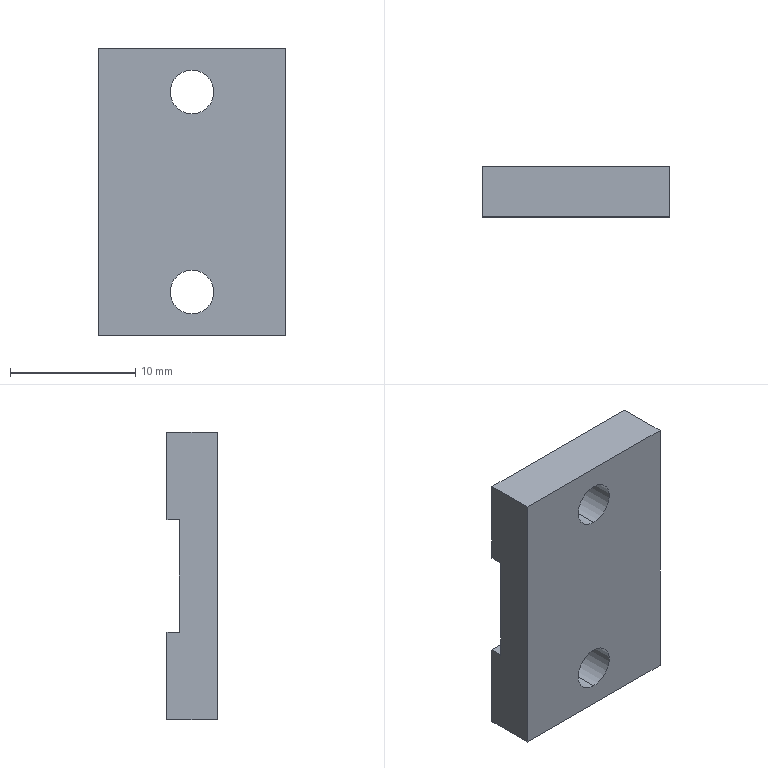Part | STEP file | 06-26 Cutter press block | 1 solid | 14 faces | box 15 x 4 x 23 mm | volume 1168 mm3 | plane 10 | cylinder 4 | commonest cylinder face diameters 3.5 x4
STEP:
#1=CARTESIAN_POINT('',(0.,0.,0.));
#2=DIRECTION('',(0.,0.,1.));
#3=DIRECTION('',(1.,0.,0.));
#4=AXIS2_PLACEMENT_3D('',#1,#2,#3);
#5=CARTESIAN_POINT('',(0.,4.,6.25));
#6=VERTEX_POINT('',#5);
#7=CARTESIAN_POINT('',(0.,0.,6.25));
#8=VERTEX_POINT('',#7);
#9=CARTESIAN_POINT('',(0.,4.,6.25));
#10=DIRECTION('',(0.,-1.,0.));
#11=VECTOR('',#10,1.);
#12=LINE('',#9,#11);
#13=CARTESIAN_POINT('',(0.,4.,8.));
#14=DIRECTION('',(0.,-1.,0.));
#15=DIRECTION('',(0.,0.,-1.));
#16=AXIS2_PLACEMENT_3D('',#13,#14,#15);
#17=CYLINDRICAL_SURFACE('',#16,1.75);
#18=CARTESIAN_POINT('',(6.283,0.));
#19=DIRECTION('',(0.,1.));
#20=VECTOR('',#19,1.);
#21=LINE('',#18,#20);
#22=(GEOMETRIC_REPRESENTATION_CONTEXT(2)PARAMETRIC_REPRESENTATION_CONTEXT()REPRESENTATION_CONTEXT('',''));
#23=DEFINITIONAL_REPRESENTATION('',(#21),#22);
#24=PCURVE('',#17,#23);
#25=CARTESIAN_POINT('',(0.,4.,8.));
#26=DIRECTION('',(0.,-1.,0.));
#27=DIRECTION('',(0.,0.,-1.));
#28=AXIS2_PLACEMENT_3D('',#25,#26,#27);
#29=CYLINDRICAL_SURFACE('',#28,1.75);
#30=CARTESIAN_POINT('',(0.,0.));
#31=DIRECTION('',(0.,1.));
#32=VECTOR('',#31,1.);
#33=LINE('',#30,#32);
#34=(GEOMETRIC_REPRESENTATION_CONTEXT(2)PARAMETRIC_REPRESENTATION_CONTEXT()REPRESENTATION_CONTEXT('',''));
#35=DEFINITIONAL_REPRESENTATION('',(#33),#34);
#36=PCURVE('',#29,#35);
#37=SURFACE_CURVE('',#12,(#24,#36),.PCURVE_S1.);
#38=EDGE_CURVE('',#6,#8,#37,.T.);
#39=ORIENTED_EDGE('',*,*,#38,.T.);
#40=CARTESIAN_POINT('',(0.,0.,9.75));
#41=VERTEX_POINT('',#40);
#42=CARTESIAN_POINT('',(0.,0.,8.));
#43=DIRECTION('',(0.,-1.,0.));
#44=DIRECTION('',(0.,0.,-1.));
#45=AXIS2_PLACEMENT_3D('',#42,#43,#44);
#46=CIRCLE('',#45,1.75);
#47=CARTESIAN_POINT('',(0.,4.));
#48=DIRECTION('',(1.,0.));
#49=VECTOR('',#48,1.);
#50=LINE('',#47,#49);
#51=(GEOMETRIC_REPRESENTATION_CONTEXT(2)PARAMETRIC_REPRESENTATION_CONTEXT()REPRESENTATION_CONTEXT('',''));
#52=DEFINITIONAL_REPRESENTATION('',(#50),#51);
#53=PCURVE('',#17,#52);
#54=CARTESIAN_POINT('',(-7.5,0.,-11.5));
#55=DIRECTION('',(0.,1.,0.));
#56=DIRECTION('',(0.,0.,1.));
#57=AXIS2_PLACEMENT_3D('',#54,#55,#56);
#58=PLANE('',#57);
#59=CARTESIAN_POINT('',(17.75,7.5));
#60=CARTESIAN_POINT('',(17.75,10.531));
#61=CARTESIAN_POINT('',(20.375,9.016));
#62=CARTESIAN_POINT('',(23.,7.5));
#63=CARTESIAN_POINT('',(20.375,5.984));
#64=CARTESIAN_POINT('',(17.75,4.469));
#65=CARTESIAN_POINT('',(17.75,7.5));
#66=(BOUNDED_CURVE()B_SPLINE_CURVE(2,(#59,#60,#61,#62,#63,#64,#65),.UNSPECIFIED.,.T.,.F.)B_SPLINE_CURVE_WITH_KNOTS((1,2,2,2,2,1),(-2.094,0.,2.094,4.189,6.283,8.378),.UNSPECIFIED.)CURVE()GEOMETRIC_REPRESENTATION_ITEM()RATIONAL_B_SPLINE_CURVE((1.,0.5,1.,0.5,1.,0.5,1.))REPRESENTATION_ITEM(''));
#67=(GEOMETRIC_REPRESENTATION_CONTEXT(2)PARAMETRIC_REPRESENTATION_CONTEXT()REPRESENTATION_CONTEXT('',''));
#68=DEFINITIONAL_REPRESENTATION('',(#66),#67);
#69=PCURVE('',#58,#68);
#70=SURFACE_CURVE('',#46,(#53,#69),.PCURVE_S1.);
#71=EDGE_CURVE('',#41,#8,#70,.T.);
#72=ORIENTED_EDGE('',*,*,#71,.F.);
#73=CARTESIAN_POINT('',(0.,4.,9.75));
#74=VERTEX_POINT('',#73);
#75=CARTESIAN_POINT('',(0.,4.,9.75));
#76=DIRECTION('',(0.,-1.,0.));
#77=VECTOR('',#76,1.);
#78=LINE('',#75,#77);
#79=CARTESIAN_POINT('',(3.142,0.));
#80=DIRECTION('',(0.,1.));
#81=VECTOR('',#80,1.);
#82=LINE('',#79,#81);
#83=(GEOMETRIC_REPRESENTATION_CONTEXT(2)PARAMETRIC_REPRESENTATION_CONTEXT()REPRESENTATION_CONTEXT('',''));
#84=DEFINITIONAL_REPRESENTATION('',(#82),#83);
#85=PCURVE('',#17,#84);
#86=CARTESIAN_POINT('',(3.142,0.));
#87=DIRECTION('',(0.,1.));
#88=VECTOR('',#87,1.);
#89=LINE('',#86,#88);
#90=(GEOMETRIC_REPRESENTATION_CONTEXT(2)PARAMETRIC_REPRESENTATION_CONTEXT()REPRESENTATION_CONTEXT('',''));
#91=DEFINITIONAL_REPRESENTATION('',(#89),#90);
#92=PCURVE('',#29,#91);
#93=SURFACE_CURVE('',#78,(#85,#92),.PCURVE_S1.);
#94=EDGE_CURVE('',#74,#41,#93,.T.);
#95=ORIENTED_EDGE('',*,*,#94,.F.);
#96=CARTESIAN_POINT('',(0.,4.,8.));
#97=DIRECTION('',(0.,1.,0.));
#98=DIRECTION('',(0.,0.,-1.));
#99=AXIS2_PLACEMENT_3D('',#96,#97,#98);
#100=CIRCLE('',#99,1.75);
#101=CARTESIAN_POINT('',(6.283,0.));
#102=DIRECTION('',(-1.,0.));
#103=VECTOR('',#102,1.);
#104=LINE('',#101,#103);
#105=(GEOMETRIC_REPRESENTATION_CONTEXT(2)PARAMETRIC_REPRESENTATION_CONTEXT()REPRESENTATION_CONTEXT('',''));
#106=DEFINITIONAL_REPRESENTATION('',(#104),#105);
#107=PCURVE('',#17,#106);
#108=CARTESIAN_POINT('',(-7.5,4.,11.5));
#109=DIRECTION('',(0.,-1.,0.));
#110=DIRECTION('',(0.,0.,-1.));
#111=AXIS2_PLACEMENT_3D('',#108,#109,#110);
#112=PLANE('',#111);
#113=CARTESIAN_POINT('',(5.25,7.5));
#114=CARTESIAN_POINT('',(5.25,4.469));
#115=CARTESIAN_POINT('',(2.625,5.984));
#116=CARTESIAN_POINT('',(0.,7.5));
#117=CARTESIAN_POINT('',(2.625,9.016));
#118=CARTESIAN_POINT('',(5.25,10.531));
#119=CARTESIAN_POINT('',(5.25,7.5));
#120=(BOUNDED_CURVE()B_SPLINE_CURVE(2,(#113,#114,#115,#116,#117,#118,#119),.UNSPECIFIED.,.T.,.F.)B_SPLINE_CURVE_WITH_KNOTS((1,2,2,2,2,1),(-2.094,0.,2.094,4.189,6.283,8.378),.UNSPECIFIED.)CURVE()GEOMETRIC_REPRESENTATION_ITEM()RATIONAL_B_SPLINE_CURVE((1.,0.5,1.,0.5,1.,0.5,1.))REPRESENTATION_ITEM(''));
#121=(GEOMETRIC_REPRESENTATION_CONTEXT(2)PARAMETRIC_REPRESENTATION_CONTEXT()REPRESENTATION_CONTEXT('',''));
#122=DEFINITIONAL_REPRESENTATION('',(#120),#121);
#123=PCURVE('',#112,#122);
#124=SURFACE_CURVE('',#100,(#107,#123),.PCURVE_S1.);
#125=EDGE_CURVE('',#6,#74,#124,.T.);
#126=ORIENTED_EDGE('',*,*,#125,.F.);
#127=EDGE_LOOP('',(#39,#72,#95,#126));
#128=FACE_BOUND('',#127,.F.);
#129=ADVANCED_FACE('',(#128),#17,.F.);
#130=CARTESIAN_POINT('',(0.,4.,-9.75));
#131=VERTEX_POINT('',#130);
#132=CARTESIAN_POINT('',(0.,0.,-9.75));
#133=VERTEX_POINT('',#132);
#134=CARTESIAN_POINT('',(0.,4.,-9.75));
#135=DIRECTION('',(0.,-1.,0.));
#136=VECTOR('',#135,1.);
#137=LINE('',#134,#136);
#138=CARTESIAN_POINT('',(0.,4.,-8.));
#139=DIRECTION('',(0.,-1.,0.));
#140=DIRECTION('',(0.,0.,-1.));
#141=AXIS2_PLACEMENT_3D('',#138,#139,#140);
#142=CYLINDRICAL_SURFACE('',#141,1.75);
#143=CARTESIAN_POINT('',(6.283,0.));
#144=DIRECTION('',(0.,1.));
#145=VECTOR('',#144,1.);
#146=LINE('',#143,#145);
#147=(GEOMETRIC_REPRESENTATION_CONTEXT(2)PARAMETRIC_REPRESENTATION_CONTEXT()REPRESENTATION_CONTEXT('',''));
#148=DEFINITIONAL_REPRESENTATION('',(#146),#147);
#149=PCURVE('',#142,#148);
#150=CARTESIAN_POINT('',(0.,4.,-8.));
#151=DIRECTION('',(0.,-1.,0.));
#152=DIRECTION('',(0.,0.,-1.));
#153=AXIS2_PLACEMENT_3D('',#150,#151,#152);
#154=CYLINDRICAL_SURFACE('',#153,1.75);
#155=CARTESIAN_POINT('',(0.,0.));
#156=DIRECTION('',(0.,1.));
#157=VECTOR('',#156,1.);
#158=LINE('',#155,#157);
#159=(GEOMETRIC_REPRESENTATION_CONTEXT(2)PARAMETRIC_REPRESENTATION_CONTEXT()REPRESENTATION_CONTEXT('',''));
#160=DEFINITIONAL_REPRESENTATION('',(#158),#159);
#161=PCURVE('',#154,#160);
#162=SURFACE_CURVE('',#137,(#149,#161),.PCURVE_S1.);
#163=EDGE_CURVE('',#131,#133,#162,.T.);
#164=ORIENTED_EDGE('',*,*,#163,.T.);
#165=CARTESIAN_POINT('',(0.,0.,-6.25));
#166=VERTEX_POINT('',#165);
#167=CARTESIAN_POINT('',(0.,0.,-8.));
#168=DIRECTION('',(0.,-1.,0.));
#169=DIRECTION('',(0.,0.,-1.));
#170=AXIS2_PLACEMENT_3D('',#167,#168,#169);
#171=CIRCLE('',#170,1.75);
#172=CARTESIAN_POINT('',(0.,4.));
#173=DIRECTION('',(1.,0.));
#174=VECTOR('',#173,1.);
#175=LINE('',#172,#174);
#176=(GEOMETRIC_REPRESENTATION_CONTEXT(2)PARAMETRIC_REPRESENTATION_CONTEXT()REPRESENTATION_CONTEXT('',''));
#177=DEFINITIONAL_REPRESENTATION('',(#175),#176);
#178=PCURVE('',#142,#177);
#179=CARTESIAN_POINT('',(1.75,7.5));
#180=CARTESIAN_POINT('',(1.75,10.531));
#181=CARTESIAN_POINT('',(4.375,9.016));
#182=CARTESIAN_POINT('',(7.,7.5));
#183=CARTESIAN_POINT('',(4.375,5.984));
#184=CARTESIAN_POINT('',(1.75,4.469));
#185=CARTESIAN_POINT('',(1.75,7.5));
#186=(BOUNDED_CURVE()B_SPLINE_CURVE(2,(#179,#180,#181,#182,#183,#184,#185),.UNSPECIFIED.,.T.,.F.)B_SPLINE_CURVE_WITH_KNOTS((1,2,2,2,2,1),(-2.094,0.,2.094,4.189,6.283,8.378),.UNSPECIFIED.)CURVE()GEOMETRIC_REPRESENTATION_ITEM()RATIONAL_B_SPLINE_CURVE((1.,0.5,1.,0.5,1.,0.5,1.))REPRESENTATION_ITEM(''));
#187=(GEOMETRIC_REPRESENTATION_CONTEXT(2)PARAMETRIC_REPRESENTATION_CONTEXT()REPRESENTATION_CONTEXT('',''));
#188=DEFINITIONAL_REPRESENTATION('',(#186),#187);
#189=PCURVE('',#58,#188);
#190=SURFACE_CURVE('',#171,(#178,#189),.PCURVE_S1.);
#191=EDGE_CURVE('',#166,#133,#190,.T.);
#192=ORIENTED_EDGE('',*,*,#191,.F.);
#193=CARTESIAN_POINT('',(0.,4.,-6.25));
#194=VERTEX_POINT('',#193);
#195=CARTESIAN_POINT('',(0.,4.,-6.25));
#196=DIRECTION('',(0.,-1.,0.));
#197=VECTOR('',#196,1.);
#198=LINE('',#195,#197);
#199=CARTESIAN_POINT('',(3.142,0.));
#200=DIRECTION('',(0.,1.));
#201=VECTOR('',#200,1.);
#202=LINE('',#199,#201);
#203=(GEOMETRIC_REPRESENTATION_CONTEXT(2)PARAMETRIC_REPRESENTATION_CONTEXT()REPRESENTATION_CONTEXT('',''));
#204=DEFINITIONAL_REPRESENTATION('',(#202),#203);
#205=PCURVE('',#142,#204);
#206=CARTESIAN_POINT('',(3.142,0.));
#207=DIRECTION('',(0.,1.));
#208=VECTOR('',#207,1.);
#209=LINE('',#206,#208);
#210=(GEOMETRIC_REPRESENTATION_CONTEXT(2)PARAMETRIC_REPRESENTATION_CONTEXT()REPRESENTATION_CONTEXT('',''));
#211=DEFINITIONAL_REPRESENTATION('',(#209),#210);
#212=PCURVE('',#154,#211);
#213=SURFACE_CURVE('',#198,(#205,#212),.PCURVE_S1.);
#214=EDGE_CURVE('',#194,#166,#213,.T.);
#215=ORIENTED_EDGE('',*,*,#214,.F.);
#216=CARTESIAN_POINT('',(0.,4.,-8.));
#217=DIRECTION('',(0.,1.,0.));
#218=DIRECTION('',(0.,0.,-1.));
#219=AXIS2_PLACEMENT_3D('',#216,#217,#218);
#220=CIRCLE('',#219,1.75);
#221=CARTESIAN_POINT('',(6.283,0.));
#222=DIRECTION('',(-1.,0.));
#223=VECTOR('',#222,1.);
#224=LINE('',#221,#223);
#225=(GEOMETRIC_REPRESENTATION_CONTEXT(2)PARAMETRIC_REPRESENTATION_CONTEXT()REPRESENTATION_CONTEXT('',''));
#226=DEFINITIONAL_REPRESENTATION('',(#224),#225);
#227=PCURVE('',#142,#226);
#228=CARTESIAN_POINT('',(-7.5,4.,-4.5));
#229=DIRECTION('',(0.,-1.,0.));
#230=DIRECTION('',(0.,0.,-1.));
#231=AXIS2_PLACEMENT_3D('',#228,#229,#230);
#232=PLANE('',#231);
#233=CARTESIAN_POINT('',(5.25,7.5));
#234=CARTESIAN_POINT('',(5.25,4.469));
#235=CARTESIAN_POINT('',(2.625,5.984));
#236=CARTESIAN_POINT('',(0.,7.5));
#237=CARTESIAN_POINT('',(2.625,9.016));
#238=CARTESIAN_POINT('',(5.25,10.531));
#239=CARTESIAN_POINT('',(5.25,7.5));
#240=(BOUNDED_CURVE()B_SPLINE_CURVE(2,(#233,#234,#235,#236,#237,#238,#239),.UNSPECIFIED.,.T.,.F.)B_SPLINE_CURVE_WITH_KNOTS((1,2,2,2,2,1),(-2.094,0.,2.094,4.189,6.283,8.378),.UNSPECIFIED.)CURVE()GEOMETRIC_REPRESENTATION_ITEM()RATIONAL_B_SPLINE_CURVE((1.,0.5,1.,0.5,1.,0.5,1.))REPRESENTATION_ITEM(''));
#241=(GEOMETRIC_REPRESENTATION_CONTEXT(2)PARAMETRIC_REPRESENTATION_CONTEXT()REPRESENTATION_CONTEXT('',''));
#242=DEFINITIONAL_REPRESENTATION('',(#240),#241);
#243=PCURVE('',#232,#242);
#244=SURFACE_CURVE('',#220,(#227,#243),.PCURVE_S1.);
#245=EDGE_CURVE('',#131,#194,#244,.T.);
#246=ORIENTED_EDGE('',*,*,#245,.F.);
#247=EDGE_LOOP('',(#164,#192,#215,#246));
#248=FACE_BOUND('',#247,.F.);
#249=ADVANCED_FACE('',(#248),#142,.F.);
#250=CARTESIAN_POINT('',(0.,0.,8.));
#251=DIRECTION('',(0.,-1.,0.));
#252=DIRECTION('',(0.,0.,-1.));
#253=AXIS2_PLACEMENT_3D('',#250,#251,#252);
#254=CIRCLE('',#253,1.75);
#255=CARTESIAN_POINT('',(0.,4.));
#256=DIRECTION('',(1.,0.));
#257=VECTOR('',#256,1.);
#258=LINE('',#255,#257);
#259=(GEOMETRIC_REPRESENTATION_CONTEXT(2)PARAMETRIC_REPRESENTATION_CONTEXT()REPRESENTATION_CONTEXT('',''));
#260=DEFINITIONAL_REPRESENTATION('',(#258),#259);
#261=PCURVE('',#29,#260);
#262=CARTESIAN_POINT('',(17.75,7.5));
#263=CARTESIAN_POINT('',(17.75,10.531));
#264=CARTESIAN_POINT('',(20.375,9.016));
#265=CARTESIAN_POINT('',(23.,7.5));
#266=CARTESIAN_POINT('',(20.375,5.984));
#267=CARTESIAN_POINT('',(17.75,4.469));
#268=CARTESIAN_POINT('',(17.75,7.5));
#269=(BOUNDED_CURVE()B_SPLINE_CURVE(2,(#262,#263,#264,#265,#266,#267,#268),.UNSPECIFIED.,.T.,.F.)B_SPLINE_CURVE_WITH_KNOTS((1,2,2,2,2,1),(-2.094,0.,2.094,4.189,6.283,8.378),.UNSPECIFIED.)CURVE()GEOMETRIC_REPRESENTATION_ITEM()RATIONAL_B_SPLINE_CURVE((1.,0.5,1.,0.5,1.,0.5,1.))REPRESENTATION_ITEM(''));
#270=(GEOMETRIC_REPRESENTATION_CONTEXT(2)PARAMETRIC_REPRESENTATION_CONTEXT()REPRESENTATION_CONTEXT('',''));
#271=DEFINITIONAL_REPRESENTATION('',(#269),#270);
#272=PCURVE('',#58,#271);
#273=SURFACE_CURVE('',#254,(#261,#272),.PCURVE_S1.);
#274=EDGE_CURVE('',#8,#41,#273,.T.);
#275=ORIENTED_EDGE('',*,*,#274,.F.);
#276=ORIENTED_EDGE('',*,*,#38,.F.);
#277=CARTESIAN_POINT('',(0.,4.,8.));
#278=DIRECTION('',(0.,1.,0.));
#279=DIRECTION('',(0.,0.,-1.));
#280=AXIS2_PLACEMENT_3D('',#277,#278,#279);
#281=CIRCLE('',#280,1.75);
#282=CARTESIAN_POINT('',(6.283,0.));
#283=DIRECTION('',(-1.,0.));
#284=VECTOR('',#283,1.);
#285=LINE('',#282,#284);
#286=(GEOMETRIC_REPRESENTATION_CONTEXT(2)PARAMETRIC_REPRESENTATION_CONTEXT()REPRESENTATION_CONTEXT('',''));
#287=DEFINITIONAL_REPRESENTATION('',(#285),#286);
#288=PCURVE('',#29,#287);
#289=CARTESIAN_POINT('',(5.25,7.5));
#290=CARTESIAN_POINT('',(5.25,4.469));
#291=CARTESIAN_POINT('',(2.625,5.984));
#292=CARTESIAN_POINT('',(0.,7.5));
#293=CARTESIAN_POINT('',(2.625,9.016));
#294=CARTESIAN_POINT('',(5.25,10.531));
#295=CARTESIAN_POINT('',(5.25,7.5));
#296=(BOUNDED_CURVE()B_SPLINE_CURVE(2,(#289,#290,#291,#292,#293,#294,#295),.UNSPECIFIED.,.T.,.F.)B_SPLINE_CURVE_WITH_KNOTS((1,2,2,2,2,1),(-2.094,0.,2.094,4.189,6.283,8.378),.UNSPECIFIED.)CURVE()GEOMETRIC_REPRESENTATION_ITEM()RATIONAL_B_SPLINE_CURVE((1.,0.5,1.,0.5,1.,0.5,1.))REPRESENTATION_ITEM(''));
#297=(GEOMETRIC_REPRESENTATION_CONTEXT(2)PARAMETRIC_REPRESENTATION_CONTEXT()REPRESENTATION_CONTEXT('',''));
#298=DEFINITIONAL_REPRESENTATION('',(#296),#297);
#299=PCURVE('',#112,#298);
#300=SURFACE_CURVE('',#281,(#288,#299),.PCURVE_S1.);
#301=EDGE_CURVE('',#74,#6,#300,.T.);
#302=ORIENTED_EDGE('',*,*,#301,.F.);
#303=ORIENTED_EDGE('',*,*,#94,.T.);
#304=EDGE_LOOP('',(#275,#276,#302,#303));
#305=FACE_BOUND('',#304,.F.);
#306=ADVANCED_FACE('',(#305),#29,.F.);
#307=CARTESIAN_POINT('',(0.,0.,-8.));
#308=DIRECTION('',(0.,-1.,0.));
#309=DIRECTION('',(0.,0.,-1.));
#310=AXIS2_PLACEMENT_3D('',#307,#308,#309);
#311=CIRCLE('',#310,1.75);
#312=CARTESIAN_POINT('',(1.75,7.5));
#313=CARTESIAN_POINT('',(1.75,10.531));
#314=CARTESIAN_POINT('',(4.375,9.016));
#315=CARTESIAN_POINT('',(7.,7.5));
#316=CARTESIAN_POINT('',(4.375,5.984));
#317=CARTESIAN_POINT('',(1.75,4.469));
#318=CARTESIAN_POINT('',(1.75,7.5));
#319=(BOUNDED_CURVE()B_SPLINE_CURVE(2,(#312,#313,#314,#315,#316,#317,#318),.UNSPECIFIED.,.T.,.F.)B_SPLINE_CURVE_WITH_KNOTS((1,2,2,2,2,1),(-2.094,0.,2.094,4.189,6.283,8.378),.UNSPECIFIED.)CURVE()GEOMETRIC_REPRESENTATION_ITEM()RATIONAL_B_SPLINE_CURVE((1.,0.5,1.,0.5,1.,0.5,1.))REPRESENTATION_ITEM(''));
#320=(GEOMETRIC_REPRESENTATION_CONTEXT(2)PARAMETRIC_REPRESENTATION_CONTEXT()REPRESENTATION_CONTEXT('',''));
#321=DEFINITIONAL_REPRESENTATION('',(#319),#320);
#322=PCURVE('',#58,#321);
#323=CARTESIAN_POINT('',(0.,4.));
#324=DIRECTION('',(1.,0.));
#325=VECTOR('',#324,1.);
#326=LINE('',#323,#325);
#327=(GEOMETRIC_REPRESENTATION_CONTEXT(2)PARAMETRIC_REPRESENTATION_CONTEXT()REPRESENTATION_CONTEXT('',''));
#328=DEFINITIONAL_REPRESENTATION('',(#326),#327);
#329=PCURVE('',#154,#328);
#330=SURFACE_CURVE('',#311,(#322,#329),.PCURVE_S1.);
#331=EDGE_CURVE('',#133,#166,#330,.T.);
#332=ORIENTED_EDGE('',*,*,#331,.F.);
#333=ORIENTED_EDGE('',*,*,#191,.F.);
#334=EDGE_LOOP('',(#332,#333));
#335=FACE_BOUND('',#334,.T.);
#336=ORIENTED_EDGE('',*,*,#274,.F.);
#337=ORIENTED_EDGE('',*,*,#71,.F.);
#338=EDGE_LOOP('',(#336,#337));
#339=FACE_BOUND('',#338,.T.);
#340=CARTESIAN_POINT('',(7.5,0.,-11.5));
#341=VERTEX_POINT('',#340);
#342=CARTESIAN_POINT('',(-7.5,0.,-11.5));
#343=VERTEX_POINT('',#342);
#344=CARTESIAN_POINT('',(0.,0.,-11.5));
#345=DIRECTION('',(-1.,0.,0.));
#346=VECTOR('',#345,1.);
#347=LINE('',#344,#346);
#348=CARTESIAN_POINT('',(0.,7.5));
#349=DIRECTION('',(0.,-1.));
#350=VECTOR('',#349,1.);
#351=LINE('',#348,#350);
#352=(GEOMETRIC_REPRESENTATION_CONTEXT(2)PARAMETRIC_REPRESENTATION_CONTEXT()REPRESENTATION_CONTEXT('',''));
#353=DEFINITIONAL_REPRESENTATION('',(#351),#352);
#354=PCURVE('',#58,#353);
#355=CARTESIAN_POINT('',(-7.5,0.,-11.5));
#356=DIRECTION('',(0.,0.,1.));
#357=DIRECTION('',(1.,0.,0.));
#358=AXIS2_PLACEMENT_3D('',#355,#356,#357);
#359=PLANE('',#358);
#360=CARTESIAN_POINT('',(7.5,0.));
#361=DIRECTION('',(-1.,0.));
#362=VECTOR('',#361,1.);
#363=LINE('',#360,#362);
#364=(GEOMETRIC_REPRESENTATION_CONTEXT(2)PARAMETRIC_REPRESENTATION_CONTEXT()REPRESENTATION_CONTEXT('',''));
#365=DEFINITIONAL_REPRESENTATION('',(#363),#364);
#366=PCURVE('',#359,#365);
#367=SURFACE_CURVE('',#347,(#354,#366),.PCURVE_S1.);
#368=EDGE_CURVE('',#341,#343,#367,.T.);
#369=ORIENTED_EDGE('',*,*,#368,.F.);
#370=CARTESIAN_POINT('',(7.5,0.,11.5));
#371=VERTEX_POINT('',#370);
#372=CARTESIAN_POINT('',(7.5,0.,0.));
#373=DIRECTION('',(0.,0.,-1.));
#374=VECTOR('',#373,1.);
#375=LINE('',#372,#374);
#376=CARTESIAN_POINT('',(11.5,15.));
#377=DIRECTION('',(-1.,0.));
#378=VECTOR('',#377,1.);
#379=LINE('',#376,#378);
#380=(GEOMETRIC_REPRESENTATION_CONTEXT(2)PARAMETRIC_REPRESENTATION_CONTEXT()REPRESENTATION_CONTEXT('',''));
#381=DEFINITIONAL_REPRESENTATION('',(#379),#380);
#382=PCURVE('',#58,#381);
#383=CARTESIAN_POINT('',(7.5,0.,11.5));
#384=DIRECTION('',(1.,0.,0.));
#385=DIRECTION('',(0.,0.,-1.));
#386=AXIS2_PLACEMENT_3D('',#383,#384,#385);
#387=PLANE('',#386);
#388=CARTESIAN_POINT('',(11.5,0.));
#389=DIRECTION('',(1.,0.));
#390=VECTOR('',#389,1.);
#391=LINE('',#388,#390);
#392=(GEOMETRIC_REPRESENTATION_CONTEXT(2)PARAMETRIC_REPRESENTATION_CONTEXT()REPRESENTATION_CONTEXT('',''));
#393=DEFINITIONAL_REPRESENTATION('',(#391),#392);
#394=PCURVE('',#387,#393);
#395=SURFACE_CURVE('',#375,(#382,#394),.PCURVE_S1.);
#396=EDGE_CURVE('',#371,#341,#395,.T.);
#397=ORIENTED_EDGE('',*,*,#396,.F.);
#398=CARTESIAN_POINT('',(-7.5,0.,11.5));
#399=VERTEX_POINT('',#398);
#400=CARTESIAN_POINT('',(0.,0.,11.5));
#401=DIRECTION('',(1.,0.,0.));
#402=VECTOR('',#401,1.);
#403=LINE('',#400,#402);
#404=CARTESIAN_POINT('',(23.,7.5));
#405=DIRECTION('',(0.,1.));
#406=VECTOR('',#405,1.);
#407=LINE('',#404,#406);
#408=(GEOMETRIC_REPRESENTATION_CONTEXT(2)PARAMETRIC_REPRESENTATION_CONTEXT()REPRESENTATION_CONTEXT('',''));
#409=DEFINITIONAL_REPRESENTATION('',(#407),#408);
#410=PCURVE('',#58,#409);
#411=CARTESIAN_POINT('',(7.5,0.,11.5));
#412=DIRECTION('',(0.,0.,-1.));
#413=DIRECTION('',(-1.,0.,0.));
#414=AXIS2_PLACEMENT_3D('',#411,#412,#413);
#415=PLANE('',#414);
#416=CARTESIAN_POINT('',(7.5,0.));
#417=DIRECTION('',(-1.,0.));
#418=VECTOR('',#417,1.);
#419=LINE('',#416,#418);
#420=(GEOMETRIC_REPRESENTATION_CONTEXT(2)PARAMETRIC_REPRESENTATION_CONTEXT()REPRESENTATION_CONTEXT('',''));
#421=DEFINITIONAL_REPRESENTATION('',(#419),#420);
#422=PCURVE('',#415,#421);
#423=SURFACE_CURVE('',#403,(#410,#422),.PCURVE_S1.);
#424=EDGE_CURVE('',#399,#371,#423,.T.);
#425=ORIENTED_EDGE('',*,*,#424,.F.);
#426=CARTESIAN_POINT('',(-7.5,0.,0.));
#427=DIRECTION('',(0.,0.,1.));
#428=VECTOR('',#427,1.);
#429=LINE('',#426,#428);
#430=CARTESIAN_POINT('',(11.5,0.));
#431=DIRECTION('',(1.,0.));
#432=VECTOR('',#431,1.);
#433=LINE('',#430,#432);
#434=(GEOMETRIC_REPRESENTATION_CONTEXT(2)PARAMETRIC_REPRESENTATION_CONTEXT()REPRESENTATION_CONTEXT('',''));
#435=DEFINITIONAL_REPRESENTATION('',(#433),#434);
#436=PCURVE('',#58,#435);
#437=CARTESIAN_POINT('',(-7.5,0.,11.5));
#438=DIRECTION('',(1.,0.,0.));
#439=DIRECTION('',(0.,0.,-1.));
#440=AXIS2_PLACEMENT_3D('',#437,#438,#439);
#441=PLANE('',#440);
#442=CARTESIAN_POINT('',(11.5,0.));
#443=DIRECTION('',(-1.,0.));
#444=VECTOR('',#443,1.);
#445=LINE('',#442,#444);
#446=(GEOMETRIC_REPRESENTATION_CONTEXT(2)PARAMETRIC_REPRESENTATION_CONTEXT()REPRESENTATION_CONTEXT('',''));
#447=DEFINITIONAL_REPRESENTATION('',(#445),#446);
#448=PCURVE('',#441,#447);
#449=SURFACE_CURVE('',#429,(#436,#448),.PCURVE_S1.);
#450=EDGE_CURVE('',#343,#399,#449,.T.);
#451=ORIENTED_EDGE('',*,*,#450,.F.);
#452=EDGE_LOOP('',(#369,#397,#425,#451));
#453=FACE_BOUND('',#452,.T.);
#454=ADVANCED_FACE('',(#335,#339,#453),#58,.F.);
#455=ORIENTED_EDGE('',*,*,#125,.F.);
#456=ORIENTED_EDGE('',*,*,#301,.F.);
#457=EDGE_LOOP('',(#455,#456));
#458=FACE_BOUND('',#457,.T.);
#459=CARTESIAN_POINT('',(7.5,4.,11.5));
#460=VERTEX_POINT('',#459);
#461=CARTESIAN_POINT('',(-7.5,4.,11.5));
#462=VERTEX_POINT('',#461);
#463=CARTESIAN_POINT('',(0.,4.,11.5));
#464=DIRECTION('',(-1.,0.,0.));
#465=VECTOR('',#464,1.);
#466=LINE('',#463,#465);
#467=CARTESIAN_POINT('',(0.,7.5));
#468=DIRECTION('',(0.,-1.));
#469=VECTOR('',#468,1.);
#470=LINE('',#467,#469);
#471=(GEOMETRIC_REPRESENTATION_CONTEXT(2)PARAMETRIC_REPRESENTATION_CONTEXT()REPRESENTATION_CONTEXT('',''));
#472=DEFINITIONAL_REPRESENTATION('',(#470),#471);
#473=PCURVE('',#112,#472);
#474=CARTESIAN_POINT('',(7.5,4.));
#475=DIRECTION('',(1.,0.));
#476=VECTOR('',#475,1.);
#477=LINE('',#474,#476);
#478=(GEOMETRIC_REPRESENTATION_CONTEXT(2)PARAMETRIC_REPRESENTATION_CONTEXT()REPRESENTATION_CONTEXT('',''));
#479=DEFINITIONAL_REPRESENTATION('',(#477),#478);
#480=PCURVE('',#415,#479);
#481=SURFACE_CURVE('',#466,(#473,#480),.PCURVE_S1.);
#482=EDGE_CURVE('',#460,#462,#481,.T.);
#483=ORIENTED_EDGE('',*,*,#482,.F.);
#484=CARTESIAN_POINT('',(7.5,4.,4.5));
#485=VERTEX_POINT('',#484);
#486=CARTESIAN_POINT('',(7.5,4.,8.));
#487=DIRECTION('',(0.,0.,1.));
#488=VECTOR('',#487,1.);
#489=LINE('',#486,#488);
#490=CARTESIAN_POINT('',(3.5,15.));
#491=DIRECTION('',(-1.,0.));
#492=VECTOR('',#491,1.);
#493=LINE('',#490,#492);
#494=(GEOMETRIC_REPRESENTATION_CONTEXT(2)PARAMETRIC_REPRESENTATION_CONTEXT()REPRESENTATION_CONTEXT('',''));
#495=DEFINITIONAL_REPRESENTATION('',(#493),#494);
#496=PCURVE('',#112,#495);
#497=CARTESIAN_POINT('',(3.5,4.));
#498=DIRECTION('',(-1.,0.));
#499=VECTOR('',#498,1.);
#500=LINE('',#497,#499);
#501=(GEOMETRIC_REPRESENTATION_CONTEXT(2)PARAMETRIC_REPRESENTATION_CONTEXT()REPRESENTATION_CONTEXT('',''));
#502=DEFINITIONAL_REPRESENTATION('',(#500),#501);
#503=PCURVE('',#387,#502);
#504=SURFACE_CURVE('',#489,(#496,#503),.PCURVE_S1.);
#505=EDGE_CURVE('',#485,#460,#504,.T.);
#506=ORIENTED_EDGE('',*,*,#505,.F.);
#507=CARTESIAN_POINT('',(-7.5,4.,4.5));
#508=VERTEX_POINT('',#507);
#509=CARTESIAN_POINT('',(0.,4.,4.5));
#510=DIRECTION('',(1.,0.,0.));
#511=VECTOR('',#510,1.);
#512=LINE('',#509,#511);
#513=CARTESIAN_POINT('',(7.,7.5));
#514=DIRECTION('',(0.,1.));
#515=VECTOR('',#514,1.);
#516=LINE('',#513,#515);
#517=(GEOMETRIC_REPRESENTATION_CONTEXT(2)PARAMETRIC_REPRESENTATION_CONTEXT()REPRESENTATION_CONTEXT('',''));
#518=DEFINITIONAL_REPRESENTATION('',(#516),#517);
#519=PCURVE('',#112,#518);
#520=CARTESIAN_POINT('',(-7.5,4.,4.5));
#521=DIRECTION('',(0.,0.,1.));
#522=DIRECTION('',(0.,-1.,0.));
#523=AXIS2_PLACEMENT_3D('',#520,#521,#522);
#524=PLANE('',#523);
#525=CARTESIAN_POINT('',(0.,7.5));
#526=DIRECTION('',(0.,1.));
#527=VECTOR('',#526,1.);
#528=LINE('',#525,#527);
#529=(GEOMETRIC_REPRESENTATION_CONTEXT(2)PARAMETRIC_REPRESENTATION_CONTEXT()REPRESENTATION_CONTEXT('',''));
#530=DEFINITIONAL_REPRESENTATION('',(#528),#529);
#531=PCURVE('',#524,#530);
#532=SURFACE_CURVE('',#512,(#519,#531),.PCURVE_S1.);
#533=EDGE_CURVE('',#508,#485,#532,.T.);
#534=ORIENTED_EDGE('',*,*,#533,.F.);
#535=CARTESIAN_POINT('',(-7.5,4.,8.));
#536=DIRECTION('',(0.,0.,-1.));
#537=VECTOR('',#536,1.);
#538=LINE('',#535,#537);
#539=CARTESIAN_POINT('',(3.5,0.));
#540=DIRECTION('',(1.,0.));
#541=VECTOR('',#540,1.);
#542=LINE('',#539,#541);
#543=(GEOMETRIC_REPRESENTATION_CONTEXT(2)PARAMETRIC_REPRESENTATION_CONTEXT()REPRESENTATION_CONTEXT('',''));
#544=DEFINITIONAL_REPRESENTATION('',(#542),#543);
#545=PCURVE('',#112,#544);
#546=CARTESIAN_POINT('',(3.5,4.));
#547=DIRECTION('',(1.,0.));
#548=VECTOR('',#547,1.);
#549=LINE('',#546,#548);
#550=(GEOMETRIC_REPRESENTATION_CONTEXT(2)PARAMETRIC_REPRESENTATION_CONTEXT()REPRESENTATION_CONTEXT('',''));
#551=DEFINITIONAL_REPRESENTATION('',(#549),#550);
#552=PCURVE('',#441,#551);
#553=SURFACE_CURVE('',#538,(#545,#552),.PCURVE_S1.);
#554=EDGE_CURVE('',#462,#508,#553,.T.);
#555=ORIENTED_EDGE('',*,*,#554,.F.);
#556=EDGE_LOOP('',(#483,#506,#534,#555));
#557=FACE_BOUND('',#556,.T.);
#558=ADVANCED_FACE('',(#458,#557),#112,.F.);
#559=ORIENTED_EDGE('',*,*,#331,.F.);
#560=ORIENTED_EDGE('',*,*,#163,.F.);
#561=CARTESIAN_POINT('',(0.,4.,-8.));
#562=DIRECTION('',(0.,1.,0.));
#563=DIRECTION('',(0.,0.,-1.));
#564=AXIS2_PLACEMENT_3D('',#561,#562,#563);
#565=CIRCLE('',#564,1.75);
#566=CARTESIAN_POINT('',(6.283,0.));
#567=DIRECTION('',(-1.,0.));
#568=VECTOR('',#567,1.);
#569=LINE('',#566,#568);
#570=(GEOMETRIC_REPRESENTATION_CONTEXT(2)PARAMETRIC_REPRESENTATION_CONTEXT()REPRESENTATION_CONTEXT('',''));
#571=DEFINITIONAL_REPRESENTATION('',(#569),#570);
#572=PCURVE('',#154,#571);
#573=CARTESIAN_POINT('',(5.25,7.5));
#574=CARTESIAN_POINT('',(5.25,4.469));
#575=CARTESIAN_POINT('',(2.625,5.984));
#576=CARTESIAN_POINT('',(0.,7.5));
#577=CARTESIAN_POINT('',(2.625,9.016));
#578=CARTESIAN_POINT('',(5.25,10.531));
#579=CARTESIAN_POINT('',(5.25,7.5));
#580=(BOUNDED_CURVE()B_SPLINE_CURVE(2,(#573,#574,#575,#576,#577,#578,#579),.UNSPECIFIED.,.T.,.F.)B_SPLINE_CURVE_WITH_KNOTS((1,2,2,2,2,1),(-2.094,0.,2.094,4.189,6.283,8.378),.UNSPECIFIED.)CURVE()GEOMETRIC_REPRESENTATION_ITEM()RATIONAL_B_SPLINE_CURVE((1.,0.5,1.,0.5,1.,0.5,1.))REPRESENTATION_ITEM(''));
#581=(GEOMETRIC_REPRESENTATION_CONTEXT(2)PARAMETRIC_REPRESENTATION_CONTEXT()REPRESENTATION_CONTEXT('',''));
#582=DEFINITIONAL_REPRESENTATION('',(#580),#581);
#583=PCURVE('',#232,#582);
#584=SURFACE_CURVE('',#565,(#572,#583),.PCURVE_S1.);
#585=EDGE_CURVE('',#194,#131,#584,.T.);
#586=ORIENTED_EDGE('',*,*,#585,.F.);
#587=ORIENTED_EDGE('',*,*,#214,.T.);
#588=EDGE_LOOP('',(#559,#560,#586,#587));
#589=FACE_BOUND('',#588,.F.);
#590=ADVANCED_FACE('',(#589),#154,.F.);
#591=ORIENTED_EDGE('',*,*,#554,.T.);
#592=CARTESIAN_POINT('',(-7.5,3.,4.5));
#593=VERTEX_POINT('',#592);
#594=CARTESIAN_POINT('',(-7.5,2.,4.5));
#595=DIRECTION('',(0.,1.,0.));
#596=VECTOR('',#595,1.);
#597=LINE('',#594,#596);
#598=CARTESIAN_POINT('',(7.,2.));
#599=DIRECTION('',(0.,1.));
#600=VECTOR('',#599,1.);
#601=LINE('',#598,#600);
#602=(GEOMETRIC_REPRESENTATION_CONTEXT(2)PARAMETRIC_REPRESENTATION_CONTEXT()REPRESENTATION_CONTEXT('',''));
#603=DEFINITIONAL_REPRESENTATION('',(#601),#602);
#604=PCURVE('',#441,#603);
#605=CARTESIAN_POINT('',(2.,0.));
#606=DIRECTION('',(-1.,0.));
#607=VECTOR('',#606,1.);
#608=LINE('',#605,#607);
#609=(GEOMETRIC_REPRESENTATION_CONTEXT(2)PARAMETRIC_REPRESENTATION_CONTEXT()REPRESENTATION_CONTEXT('',''));
#610=DEFINITIONAL_REPRESENTATION('',(#608),#609);
#611=PCURVE('',#524,#610);
#612=SURFACE_CURVE('',#597,(#604,#611),.PCURVE_S1.);
#613=EDGE_CURVE('',#593,#508,#612,.T.);
#614=ORIENTED_EDGE('',*,*,#613,.F.);
#615=CARTESIAN_POINT('',(-7.5,3.,-4.5));
#616=VERTEX_POINT('',#615);
#617=CARTESIAN_POINT('',(-7.5,3.,0.));
#618=DIRECTION('',(0.,0.,1.));
#619=VECTOR('',#618,1.);
#620=LINE('',#617,#619);
#621=CARTESIAN_POINT('',(11.5,3.));
#622=DIRECTION('',(-1.,0.));
#623=VECTOR('',#622,1.);
#624=LINE('',#621,#623);
#625=(GEOMETRIC_REPRESENTATION_CONTEXT(2)PARAMETRIC_REPRESENTATION_CONTEXT()REPRESENTATION_CONTEXT('',''));
#626=DEFINITIONAL_REPRESENTATION('',(#624),#625);
#627=PCURVE('',#441,#626);
#628=CARTESIAN_POINT('',(-7.5,3.,4.5));
#629=DIRECTION('',(0.,-1.,0.));
#630=DIRECTION('',(0.,0.,-1.));
#631=AXIS2_PLACEMENT_3D('',#628,#629,#630);
#632=PLANE('',#631);
#633=CARTESIAN_POINT('',(4.5,0.));
#634=DIRECTION('',(-1.,0.));
#635=VECTOR('',#634,1.);
#636=LINE('',#633,#635);
#637=(GEOMETRIC_REPRESENTATION_CONTEXT(2)PARAMETRIC_REPRESENTATION_CONTEXT()REPRESENTATION_CONTEXT('',''));
#638=DEFINITIONAL_REPRESENTATION('',(#636),#637);
#639=PCURVE('',#632,#638);
#640=SURFACE_CURVE('',#620,(#627,#639),.PCURVE_S1.);
#641=EDGE_CURVE('',#616,#593,#640,.T.);
#642=ORIENTED_EDGE('',*,*,#641,.F.);
#643=CARTESIAN_POINT('',(-7.5,4.,-4.5));
#644=VERTEX_POINT('',#643);
#645=CARTESIAN_POINT('',(-7.5,3.5,-4.5));
#646=DIRECTION('',(0.,1.,0.));
#647=VECTOR('',#646,1.);
#648=LINE('',#645,#647);
#649=CARTESIAN_POINT('',(16.,3.5));
#650=DIRECTION('',(0.,1.));
#651=VECTOR('',#650,1.);
#652=LINE('',#649,#651);
#653=(GEOMETRIC_REPRESENTATION_CONTEXT(2)PARAMETRIC_REPRESENTATION_CONTEXT()REPRESENTATION_CONTEXT('',''));
#654=DEFINITIONAL_REPRESENTATION('',(#652),#653);
#655=PCURVE('',#441,#654);
#656=CARTESIAN_POINT('',(7.5,3.,-4.5));
#657=DIRECTION('',(0.,0.,-1.));
#658=DIRECTION('',(-1.,0.,0.));
#659=AXIS2_PLACEMENT_3D('',#656,#657,#658);
#660=PLANE('',#659);
#661=CARTESIAN_POINT('',(15.,0.5));
#662=DIRECTION('',(0.,1.));
#663=VECTOR('',#662,1.);
#664=LINE('',#661,#663);
#665=(GEOMETRIC_REPRESENTATION_CONTEXT(2)PARAMETRIC_REPRESENTATION_CONTEXT()REPRESENTATION_CONTEXT('',''));
#666=DEFINITIONAL_REPRESENTATION('',(#664),#665);
#667=PCURVE('',#660,#666);
#668=SURFACE_CURVE('',#648,(#655,#667),.PCURVE_S1.);
#669=EDGE_CURVE('',#616,#644,#668,.T.);
#670=ORIENTED_EDGE('',*,*,#669,.T.);
#671=CARTESIAN_POINT('',(-7.5,4.,-11.5));
#672=VERTEX_POINT('',#671);
#673=CARTESIAN_POINT('',(-7.5,4.,0.));
#674=DIRECTION('',(0.,0.,1.));
#675=VECTOR('',#674,1.);
#676=LINE('',#673,#675);
#677=CARTESIAN_POINT('',(11.5,4.));
#678=DIRECTION('',(-1.,0.));
#679=VECTOR('',#678,1.);
#680=LINE('',#677,#679);
#681=(GEOMETRIC_REPRESENTATION_CONTEXT(2)PARAMETRIC_REPRESENTATION_CONTEXT()REPRESENTATION_CONTEXT('',''));
#682=DEFINITIONAL_REPRESENTATION('',(#680),#681);
#683=PCURVE('',#441,#682);
#684=CARTESIAN_POINT('',(-4.5,0.));
#685=DIRECTION('',(-1.,0.));
#686=VECTOR('',#685,1.);
#687=LINE('',#684,#686);
#688=(GEOMETRIC_REPRESENTATION_CONTEXT(2)PARAMETRIC_REPRESENTATION_CONTEXT()REPRESENTATION_CONTEXT('',''));
#689=DEFINITIONAL_REPRESENTATION('',(#687),#688);
#690=PCURVE('',#232,#689);
#691=SURFACE_CURVE('',#676,(#683,#690),.PCURVE_S1.);
#692=EDGE_CURVE('',#672,#644,#691,.T.);
#693=ORIENTED_EDGE('',*,*,#692,.F.);
#694=CARTESIAN_POINT('',(-7.5,2.,-11.5));
#695=DIRECTION('',(0.,1.,0.));
#696=VECTOR('',#695,1.);
#697=LINE('',#694,#696);
#698=CARTESIAN_POINT('',(23.,2.));
#699=DIRECTION('',(0.,1.));
#700=VECTOR('',#699,1.);
#701=LINE('',#698,#700);
#702=(GEOMETRIC_REPRESENTATION_CONTEXT(2)PARAMETRIC_REPRESENTATION_CONTEXT()REPRESENTATION_CONTEXT('',''));
#703=DEFINITIONAL_REPRESENTATION('',(#701),#702);
#704=PCURVE('',#441,#703);
#705=CARTESIAN_POINT('',(0.,2.));
#706=DIRECTION('',(0.,1.));
#707=VECTOR('',#706,1.);
#708=LINE('',#705,#707);
#709=(GEOMETRIC_REPRESENTATION_CONTEXT(2)PARAMETRIC_REPRESENTATION_CONTEXT()REPRESENTATION_CONTEXT('',''));
#710=DEFINITIONAL_REPRESENTATION('',(#708),#709);
#711=PCURVE('',#359,#710);
#712=SURFACE_CURVE('',#697,(#704,#711),.PCURVE_S1.);
#713=EDGE_CURVE('',#343,#672,#712,.T.);
#714=ORIENTED_EDGE('',*,*,#713,.F.);
#715=ORIENTED_EDGE('',*,*,#450,.T.);
#716=CARTESIAN_POINT('',(-7.5,2.,11.5));
#717=DIRECTION('',(0.,-1.,0.));
#718=VECTOR('',#717,1.);
#719=LINE('',#716,#718);
#720=CARTESIAN_POINT('',(0.,2.));
#721=DIRECTION('',(0.,-1.));
#722=VECTOR('',#721,1.);
#723=LINE('',#720,#722);
#724=(GEOMETRIC_REPRESENTATION_CONTEXT(2)PARAMETRIC_REPRESENTATION_CONTEXT()REPRESENTATION_CONTEXT('',''));
#725=DEFINITIONAL_REPRESENTATION('',(#723),#724);
#726=PCURVE('',#441,#725);
#727=CARTESIAN_POINT('',(15.,2.));
#728=DIRECTION('',(0.,-1.));
#729=VECTOR('',#728,1.);
#730=LINE('',#727,#729);
#731=(GEOMETRIC_REPRESENTATION_CONTEXT(2)PARAMETRIC_REPRESENTATION_CONTEXT()REPRESENTATION_CONTEXT('',''));
#732=DEFINITIONAL_REPRESENTATION('',(#730),#731);
#733=PCURVE('',#415,#732);
#734=SURFACE_CURVE('',#719,(#726,#733),.PCURVE_S1.);
#735=EDGE_CURVE('',#462,#399,#734,.T.);
#736=ORIENTED_EDGE('',*,*,#735,.F.);
#737=EDGE_LOOP('',(#591,#614,#642,#670,#693,#714,#715,#736));
#738=FACE_BOUND('',#737,.T.);
#739=ADVANCED_FACE('',(#738),#441,.F.);
#740=CARTESIAN_POINT('',(7.5,4.,-11.5));
#741=VERTEX_POINT('',#740);
#742=CARTESIAN_POINT('',(0.,4.,-11.5));
#743=DIRECTION('',(-1.,0.,0.));
#744=VECTOR('',#743,1.);
#745=LINE('',#742,#744);
#746=CARTESIAN_POINT('',(7.5,4.));
#747=DIRECTION('',(-1.,0.));
#748=VECTOR('',#747,1.);
#749=LINE('',#746,#748);
#750=(GEOMETRIC_REPRESENTATION_CONTEXT(2)PARAMETRIC_REPRESENTATION_CONTEXT()REPRESENTATION_CONTEXT('',''));
#751=DEFINITIONAL_REPRESENTATION('',(#749),#750);
#752=PCURVE('',#359,#751);
#753=CARTESIAN_POINT('',(7.,7.5));
#754=DIRECTION('',(0.,-1.));
#755=VECTOR('',#754,1.);
#756=LINE('',#753,#755);
#757=(GEOMETRIC_REPRESENTATION_CONTEXT(2)PARAMETRIC_REPRESENTATION_CONTEXT()REPRESENTATION_CONTEXT('',''));
#758=DEFINITIONAL_REPRESENTATION('',(#756),#757);
#759=PCURVE('',#232,#758);
#760=SURFACE_CURVE('',#745,(#752,#759),.PCURVE_S1.);
#761=EDGE_CURVE('',#741,#672,#760,.T.);
#762=ORIENTED_EDGE('',*,*,#761,.F.);
#763=CARTESIAN_POINT('',(7.5,2.,-11.5));
#764=DIRECTION('',(0.,1.,0.));
#765=VECTOR('',#764,1.);
#766=LINE('',#763,#765);
#767=CARTESIAN_POINT('',(15.,2.));
#768=DIRECTION('',(0.,1.));
#769=VECTOR('',#768,1.);
#770=LINE('',#767,#769);
#771=(GEOMETRIC_REPRESENTATION_CONTEXT(2)PARAMETRIC_REPRESENTATION_CONTEXT()REPRESENTATION_CONTEXT('',''));
#772=DEFINITIONAL_REPRESENTATION('',(#770),#771);
#773=PCURVE('',#359,#772);
#774=CARTESIAN_POINT('',(23.,2.));
#775=DIRECTION('',(0.,1.));
#776=VECTOR('',#775,1.);
#777=LINE('',#774,#776);
#778=(GEOMETRIC_REPRESENTATION_CONTEXT(2)PARAMETRIC_REPRESENTATION_CONTEXT()REPRESENTATION_CONTEXT('',''));
#779=DEFINITIONAL_REPRESENTATION('',(#777),#778);
#780=PCURVE('',#387,#779);
#781=SURFACE_CURVE('',#766,(#773,#780),.PCURVE_S1.);
#782=EDGE_CURVE('',#341,#741,#781,.T.);
#783=ORIENTED_EDGE('',*,*,#782,.F.);
#784=ORIENTED_EDGE('',*,*,#368,.T.);
#785=ORIENTED_EDGE('',*,*,#713,.T.);
#786=EDGE_LOOP('',(#762,#783,#784,#785));
#787=FACE_BOUND('',#786,.T.);
#788=ADVANCED_FACE('',(#787),#359,.F.);
#789=CARTESIAN_POINT('',(7.5,3.,4.5));
#790=VERTEX_POINT('',#789);
#791=CARTESIAN_POINT('',(7.5,2.,4.5));
#792=DIRECTION('',(0.,1.,0.));
#793=VECTOR('',#792,1.);
#794=LINE('',#791,#793);
#795=CARTESIAN_POINT('',(7.,2.));
#796=DIRECTION('',(0.,1.));
#797=VECTOR('',#796,1.);
#798=LINE('',#795,#797);
#799=(GEOMETRIC_REPRESENTATION_CONTEXT(2)PARAMETRIC_REPRESENTATION_CONTEXT()REPRESENTATION_CONTEXT('',''));
#800=DEFINITIONAL_REPRESENTATION('',(#798),#799);
#801=PCURVE('',#387,#800);
#802=CARTESIAN_POINT('',(2.,15.));
#803=DIRECTION('',(-1.,0.));
#804=VECTOR('',#803,1.);
#805=LINE('',#802,#804);
#806=(GEOMETRIC_REPRESENTATION_CONTEXT(2)PARAMETRIC_REPRESENTATION_CONTEXT()REPRESENTATION_CONTEXT('',''));
#807=DEFINITIONAL_REPRESENTATION('',(#805),#806);
#808=PCURVE('',#524,#807);
#809=SURFACE_CURVE('',#794,(#801,#808),.PCURVE_S1.);
#810=EDGE_CURVE('',#790,#485,#809,.T.);
#811=ORIENTED_EDGE('',*,*,#810,.T.);
#812=ORIENTED_EDGE('',*,*,#505,.T.);
#813=CARTESIAN_POINT('',(7.5,2.,11.5));
#814=DIRECTION('',(0.,-1.,0.));
#815=VECTOR('',#814,1.);
#816=LINE('',#813,#815);
#817=CARTESIAN_POINT('',(0.,2.));
#818=DIRECTION('',(0.,-1.));
#819=VECTOR('',#818,1.);
#820=LINE('',#817,#819);
#821=(GEOMETRIC_REPRESENTATION_CONTEXT(2)PARAMETRIC_REPRESENTATION_CONTEXT()REPRESENTATION_CONTEXT('',''));
#822=DEFINITIONAL_REPRESENTATION('',(#820),#821);
#823=PCURVE('',#387,#822);
#824=CARTESIAN_POINT('',(0.,2.));
#825=DIRECTION('',(0.,-1.));
#826=VECTOR('',#825,1.);
#827=LINE('',#824,#826);
#828=(GEOMETRIC_REPRESENTATION_CONTEXT(2)PARAMETRIC_REPRESENTATION_CONTEXT()REPRESENTATION_CONTEXT('',''));
#829=DEFINITIONAL_REPRESENTATION('',(#827),#828);
#830=PCURVE('',#415,#829);
#831=SURFACE_CURVE('',#816,(#823,#830),.PCURVE_S1.);
#832=EDGE_CURVE('',#460,#371,#831,.T.);
#833=ORIENTED_EDGE('',*,*,#832,.T.);
#834=ORIENTED_EDGE('',*,*,#396,.T.);
#835=ORIENTED_EDGE('',*,*,#782,.T.);
#836=CARTESIAN_POINT('',(7.5,4.,-4.5));
#837=VERTEX_POINT('',#836);
#838=CARTESIAN_POINT('',(7.5,4.,0.));
#839=DIRECTION('',(0.,0.,1.));
#840=VECTOR('',#839,1.);
#841=LINE('',#838,#840);
#842=CARTESIAN_POINT('',(11.5,4.));
#843=DIRECTION('',(-1.,0.));
#844=VECTOR('',#843,1.);
#845=LINE('',#842,#844);
#846=(GEOMETRIC_REPRESENTATION_CONTEXT(2)PARAMETRIC_REPRESENTATION_CONTEXT()REPRESENTATION_CONTEXT('',''));
#847=DEFINITIONAL_REPRESENTATION('',(#845),#846);
#848=PCURVE('',#387,#847);
#849=CARTESIAN_POINT('',(-4.5,15.));
#850=DIRECTION('',(-1.,0.));
#851=VECTOR('',#850,1.);
#852=LINE('',#849,#851);
#853=(GEOMETRIC_REPRESENTATION_CONTEXT(2)PARAMETRIC_REPRESENTATION_CONTEXT()REPRESENTATION_CONTEXT('',''));
#854=DEFINITIONAL_REPRESENTATION('',(#852),#853);
#855=PCURVE('',#232,#854);
#856=SURFACE_CURVE('',#841,(#848,#855),.PCURVE_S1.);
#857=EDGE_CURVE('',#741,#837,#856,.T.);
#858=ORIENTED_EDGE('',*,*,#857,.T.);
#859=CARTESIAN_POINT('',(7.5,3.,-4.5));
#860=VERTEX_POINT('',#859);
#861=CARTESIAN_POINT('',(7.5,3.5,-4.5));
#862=DIRECTION('',(0.,-1.,0.));
#863=VECTOR('',#862,1.);
#864=LINE('',#861,#863);
#865=CARTESIAN_POINT('',(16.,3.5));
#866=DIRECTION('',(0.,-1.));
#867=VECTOR('',#866,1.);
#868=LINE('',#865,#867);
#869=(GEOMETRIC_REPRESENTATION_CONTEXT(2)PARAMETRIC_REPRESENTATION_CONTEXT()REPRESENTATION_CONTEXT('',''));
#870=DEFINITIONAL_REPRESENTATION('',(#868),#869);
#871=PCURVE('',#387,#870);
#872=CARTESIAN_POINT('',(0.,0.5));
#873=DIRECTION('',(0.,-1.));
#874=VECTOR('',#873,1.);
#875=LINE('',#872,#874);
#876=(GEOMETRIC_REPRESENTATION_CONTEXT(2)PARAMETRIC_REPRESENTATION_CONTEXT()REPRESENTATION_CONTEXT('',''));
#877=DEFINITIONAL_REPRESENTATION('',(#875),#876);
#878=PCURVE('',#660,#877);
#879=SURFACE_CURVE('',#864,(#871,#878),.PCURVE_S1.);
#880=EDGE_CURVE('',#837,#860,#879,.T.);
#881=ORIENTED_EDGE('',*,*,#880,.T.);
#882=CARTESIAN_POINT('',(7.5,3.,0.));
#883=DIRECTION('',(0.,0.,1.));
#884=VECTOR('',#883,1.);
#885=LINE('',#882,#884);
#886=CARTESIAN_POINT('',(11.5,3.));
#887=DIRECTION('',(-1.,0.));
#888=VECTOR('',#887,1.);
#889=LINE('',#886,#888);
#890=(GEOMETRIC_REPRESENTATION_CONTEXT(2)PARAMETRIC_REPRESENTATION_CONTEXT()REPRESENTATION_CONTEXT('',''));
#891=DEFINITIONAL_REPRESENTATION('',(#889),#890);
#892=PCURVE('',#387,#891);
#893=CARTESIAN_POINT('',(4.5,15.));
#894=DIRECTION('',(-1.,0.));
#895=VECTOR('',#894,1.);
#896=LINE('',#893,#895);
#897=(GEOMETRIC_REPRESENTATION_CONTEXT(2)PARAMETRIC_REPRESENTATION_CONTEXT()REPRESENTATION_CONTEXT('',''));
#898=DEFINITIONAL_REPRESENTATION('',(#896),#897);
#899=PCURVE('',#632,#898);
#900=SURFACE_CURVE('',#885,(#892,#899),.PCURVE_S1.);
#901=EDGE_CURVE('',#860,#790,#900,.T.);
#902=ORIENTED_EDGE('',*,*,#901,.T.);
#903=EDGE_LOOP('',(#811,#812,#833,#834,#835,#858,#881,#902));
#904=FACE_BOUND('',#903,.T.);
#905=ADVANCED_FACE('',(#904),#387,.T.);
#906=ORIENTED_EDGE('',*,*,#424,.T.);
#907=ORIENTED_EDGE('',*,*,#832,.F.);
#908=ORIENTED_EDGE('',*,*,#482,.T.);
#909=ORIENTED_EDGE('',*,*,#735,.T.);
#910=EDGE_LOOP('',(#906,#907,#908,#909));
#911=FACE_BOUND('',#910,.T.);
#912=ADVANCED_FACE('',(#911),#415,.F.);
#913=ORIENTED_EDGE('',*,*,#533,.T.);
#914=ORIENTED_EDGE('',*,*,#810,.F.);
#915=CARTESIAN_POINT('',(0.,3.,4.5));
#916=DIRECTION('',(1.,0.,0.));
#917=VECTOR('',#916,1.);
#918=LINE('',#915,#917);
#919=CARTESIAN_POINT('',(1.,7.5));
#920=DIRECTION('',(0.,1.));
#921=VECTOR('',#920,1.);
#922=LINE('',#919,#921);
#923=(GEOMETRIC_REPRESENTATION_CONTEXT(2)PARAMETRIC_REPRESENTATION_CONTEXT()REPRESENTATION_CONTEXT('',''));
#924=DEFINITIONAL_REPRESENTATION('',(#922),#923);
#925=PCURVE('',#524,#924);
#926=CARTESIAN_POINT('',(0.,7.5));
#927=DIRECTION('',(0.,1.));
#928=VECTOR('',#927,1.);
#929=LINE('',#926,#928);
#930=(GEOMETRIC_REPRESENTATION_CONTEXT(2)PARAMETRIC_REPRESENTATION_CONTEXT()REPRESENTATION_CONTEXT('',''));
#931=DEFINITIONAL_REPRESENTATION('',(#929),#930);
#932=PCURVE('',#632,#931);
#933=SURFACE_CURVE('',#918,(#925,#932),.PCURVE_S1.);
#934=EDGE_CURVE('',#593,#790,#933,.T.);
#935=ORIENTED_EDGE('',*,*,#934,.F.);
#936=ORIENTED_EDGE('',*,*,#613,.T.);
#937=EDGE_LOOP('',(#913,#914,#935,#936));
#938=FACE_BOUND('',#937,.T.);
#939=ADVANCED_FACE('',(#938),#524,.F.);
#940=ORIENTED_EDGE('',*,*,#245,.F.);
#941=ORIENTED_EDGE('',*,*,#585,.F.);
#942=EDGE_LOOP('',(#940,#941));
#943=FACE_BOUND('',#942,.T.);
#944=CARTESIAN_POINT('',(0.,4.,-4.5));
#945=DIRECTION('',(-1.,0.,0.));
#946=VECTOR('',#945,1.);
#947=LINE('',#944,#946);
#948=CARTESIAN_POINT('',(0.,7.5));
#949=DIRECTION('',(0.,-1.));
#950=VECTOR('',#949,1.);
#951=LINE('',#948,#950);
#952=(GEOMETRIC_REPRESENTATION_CONTEXT(2)PARAMETRIC_REPRESENTATION_CONTEXT()REPRESENTATION_CONTEXT('',''));
#953=DEFINITIONAL_REPRESENTATION('',(#951),#952);
#954=PCURVE('',#232,#953);
#955=CARTESIAN_POINT('',(7.5,1.));
#956=DIRECTION('',(1.,0.));
#957=VECTOR('',#956,1.);
#958=LINE('',#955,#957);
#959=(GEOMETRIC_REPRESENTATION_CONTEXT(2)PARAMETRIC_REPRESENTATION_CONTEXT()REPRESENTATION_CONTEXT('',''));
#960=DEFINITIONAL_REPRESENTATION('',(#958),#959);
#961=PCURVE('',#660,#960);
#962=SURFACE_CURVE('',#947,(#954,#961),.PCURVE_S1.);
#963=EDGE_CURVE('',#837,#644,#962,.T.);
#964=ORIENTED_EDGE('',*,*,#963,.F.);
#965=ORIENTED_EDGE('',*,*,#857,.F.);
#966=ORIENTED_EDGE('',*,*,#761,.T.);
#967=ORIENTED_EDGE('',*,*,#692,.T.);
#968=EDGE_LOOP('',(#964,#965,#966,#967));
#969=FACE_BOUND('',#968,.T.);
#970=ADVANCED_FACE('',(#943,#969),#232,.F.);
#971=ORIENTED_EDGE('',*,*,#934,.T.);
#972=ORIENTED_EDGE('',*,*,#901,.F.);
#973=CARTESIAN_POINT('',(0.,3.,-4.5));
#974=DIRECTION('',(1.,0.,0.));
#975=VECTOR('',#974,1.);
#976=LINE('',#973,#975);
#977=CARTESIAN_POINT('',(9.,7.5));
#978=DIRECTION('',(0.,1.));
#979=VECTOR('',#978,1.);
#980=LINE('',#977,#979);
#981=(GEOMETRIC_REPRESENTATION_CONTEXT(2)PARAMETRIC_REPRESENTATION_CONTEXT()REPRESENTATION_CONTEXT('',''));
#982=DEFINITIONAL_REPRESENTATION('',(#980),#981);
#983=PCURVE('',#632,#982);
#984=CARTESIAN_POINT('',(7.5,0.));
#985=DIRECTION('',(-1.,0.));
#986=VECTOR('',#985,1.);
#987=LINE('',#984,#986);
#988=(GEOMETRIC_REPRESENTATION_CONTEXT(2)PARAMETRIC_REPRESENTATION_CONTEXT()REPRESENTATION_CONTEXT('',''));
#989=DEFINITIONAL_REPRESENTATION('',(#987),#988);
#990=PCURVE('',#660,#989);
#991=SURFACE_CURVE('',#976,(#983,#990),.PCURVE_S1.);
#992=EDGE_CURVE('',#616,#860,#991,.T.);
#993=ORIENTED_EDGE('',*,*,#992,.F.);
#994=ORIENTED_EDGE('',*,*,#641,.T.);
#995=EDGE_LOOP('',(#971,#972,#993,#994));
#996=FACE_BOUND('',#995,.T.);
#997=ADVANCED_FACE('',(#996),#632,.F.);
#998=ORIENTED_EDGE('',*,*,#992,.T.);
#999=ORIENTED_EDGE('',*,*,#880,.F.);
#1000=ORIENTED_EDGE('',*,*,#963,.T.);
#1001=ORIENTED_EDGE('',*,*,#669,.F.);
#1002=EDGE_LOOP('',(#998,#999,#1000,#1001));
#1003=FACE_BOUND('',#1002,.T.);
#1004=ADVANCED_FACE('',(#1003),#660,.F.);
#1005=CLOSED_SHELL('',(#129,#249,#306,#454,#558,#590,#739,#788,#905,#912,#939,#970,#997,#1004));
#1006=MANIFOLD_SOLID_BREP('',#1005);
#1007=(LENGTH_UNIT()NAMED_UNIT(*)SI_UNIT(.MILLI.,.METRE.));
#1008=UNCERTAINTY_MEASURE_WITH_UNIT(LENGTH_MEASURE(0.0000001),#1007,'','');
#1009=(NAMED_UNIT(*)PLANE_ANGLE_UNIT()SI_UNIT($,.RADIAN.));
#1010=(NAMED_UNIT(*)SI_UNIT($,.STERADIAN.)SOLID_ANGLE_UNIT());
#1011=(GEOMETRIC_REPRESENTATION_CONTEXT(3)GLOBAL_UNCERTAINTY_ASSIGNED_CONTEXT((#1008))GLOBAL_UNIT_ASSIGNED_CONTEXT((#1007,#1009,#1010))REPRESENTATION_CONTEXT('',''));
#1012=ADVANCED_BREP_SHAPE_REPRESENTATION('',(#4,#1006),#1011);